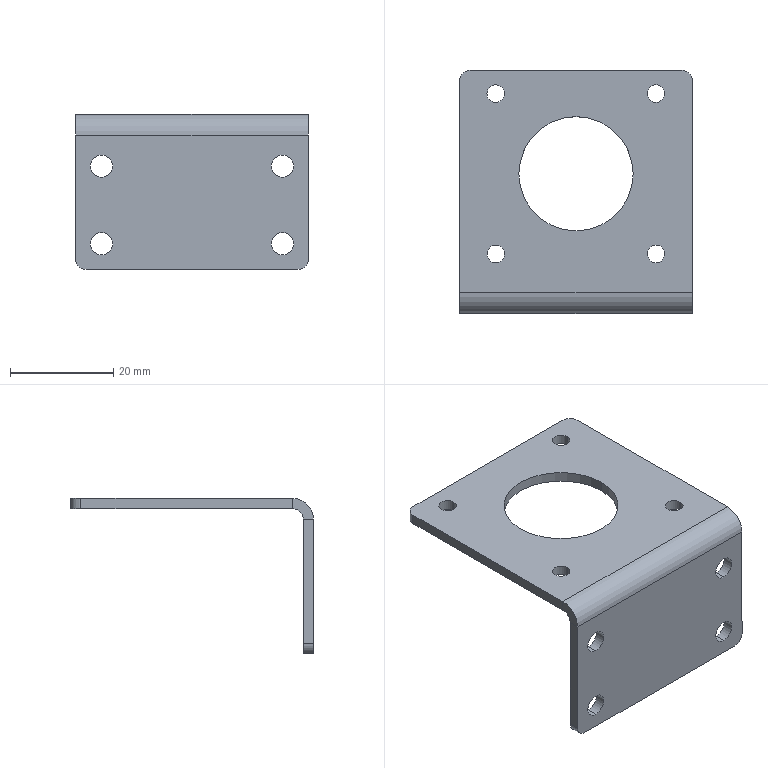Part | SolidWorks | features 3DProfileFeature 2, HoleWzd 2, EdgeFlange 1, Fillet 1, FlatPattern 1, ICE 1, SMBaseFlange 1, SheetMetal 1 | 1 solid | 36 faces | box 45 x 47 x 30 mm | volume 5671 mm3 | cylinder 24 | plane 12 | commonest cylinder face diameters 3.4 x8 4.3 x8 4 x5 22.1 x2 8 x1
STEP:
#1=CARTESIAN_POINT('',(-17.5,-23.5,-27.15));
#2=VERTEX_POINT('',#1);
#3=CARTESIAN_POINT('',(-17.5,-23.5,-22.85));
#4=VERTEX_POINT('',#3);
#5=CARTESIAN_POINT('',(-17.5,-23.5,-25.));
#6=DIRECTION('',(0.,1.,0.));
#7=DIRECTION('',(0.,0.,1.));
#8=AXIS2_PLACEMENT_3D('',#5,#6,#7);
#9=CIRCLE('',#8,2.15);
#10=EDGE_CURVE('',#2,#4,#9,.T.);
#11=ORIENTED_EDGE('',*,*,#10,.F.);
#12=CARTESIAN_POINT('',(-17.5,-21.5,-27.15));
#13=VERTEX_POINT('',#12);
#14=CARTESIAN_POINT('',(-17.5,-21.5,-27.15));
#15=DIRECTION('',(0.,1.,0.));
#16=VECTOR('',#15,1000.);
#17=LINE('',#14,#16);
#18=EDGE_CURVE('',#2,#13,#17,.T.);
#19=ORIENTED_EDGE('',*,*,#18,.T.);
#20=CARTESIAN_POINT('',(-17.5,-21.5,-22.85));
#21=VERTEX_POINT('',#20);
#22=CARTESIAN_POINT('',(-17.5,-21.5,-25.));
#23=DIRECTION('',(0.,1.,0.));
#24=DIRECTION('',(0.,0.,1.));
#25=AXIS2_PLACEMENT_3D('',#22,#23,#24);
#26=CIRCLE('',#25,2.15);
#27=EDGE_CURVE('',#13,#21,#26,.T.);
#28=ORIENTED_EDGE('',*,*,#27,.T.);
#29=CARTESIAN_POINT('',(-17.5,-21.5,-22.85));
#30=DIRECTION('',(0.,1.,0.));
#31=VECTOR('',#30,1000.);
#32=LINE('',#29,#31);
#33=EDGE_CURVE('',#4,#21,#32,.T.);
#34=ORIENTED_EDGE('',*,*,#33,.F.);
#35=EDGE_LOOP('',(#11,#19,#28,#34));
#36=FACE_OUTER_BOUND('',#35,.T.);
#37=CARTESIAN_POINT('',(-17.5,-21.5,-25.));
#38=DIRECTION('',(0.,1.,0.));
#39=DIRECTION('',(0.,0.,1.));
#40=AXIS2_PLACEMENT_3D('',#37,#38,#39);
#41=CYLINDRICAL_SURFACE('',#40,2.15);
#42=ADVANCED_FACE('',(#36),#41,.F.);
#43=CARTESIAN_POINT('',(-17.5,-23.5,-12.15));
#44=VERTEX_POINT('',#43);
#45=CARTESIAN_POINT('',(-17.5,-23.5,-7.85));
#46=VERTEX_POINT('',#45);
#47=CARTESIAN_POINT('',(-17.5,-23.5,-10.));
#48=DIRECTION('',(0.,1.,0.));
#49=DIRECTION('',(0.,0.,1.));
#50=AXIS2_PLACEMENT_3D('',#47,#48,#49);
#51=CIRCLE('',#50,2.15);
#52=EDGE_CURVE('',#44,#46,#51,.T.);
#53=ORIENTED_EDGE('',*,*,#52,.F.);
#54=CARTESIAN_POINT('',(-17.5,-21.5,-12.15));
#55=VERTEX_POINT('',#54);
#56=CARTESIAN_POINT('',(-17.5,-21.5,-12.15));
#57=DIRECTION('',(0.,1.,0.));
#58=VECTOR('',#57,1000.);
#59=LINE('',#56,#58);
#60=EDGE_CURVE('',#44,#55,#59,.T.);
#61=ORIENTED_EDGE('',*,*,#60,.T.);
#62=CARTESIAN_POINT('',(-17.5,-21.5,-7.85));
#63=VERTEX_POINT('',#62);
#64=CARTESIAN_POINT('',(-17.5,-21.5,-10.));
#65=DIRECTION('',(0.,1.,0.));
#66=DIRECTION('',(0.,0.,1.));
#67=AXIS2_PLACEMENT_3D('',#64,#65,#66);
#68=CIRCLE('',#67,2.15);
#69=EDGE_CURVE('',#55,#63,#68,.T.);
#70=ORIENTED_EDGE('',*,*,#69,.T.);
#71=CARTESIAN_POINT('',(-17.5,-21.5,-7.85));
#72=DIRECTION('',(0.,1.,0.));
#73=VECTOR('',#72,1000.);
#74=LINE('',#71,#73);
#75=EDGE_CURVE('',#46,#63,#74,.T.);
#76=ORIENTED_EDGE('',*,*,#75,.F.);
#77=EDGE_LOOP('',(#53,#61,#70,#76));
#78=FACE_OUTER_BOUND('',#77,.T.);
#79=CARTESIAN_POINT('',(-17.5,-21.5,-10.));
#80=DIRECTION('',(0.,1.,0.));
#81=DIRECTION('',(0.,0.,1.));
#82=AXIS2_PLACEMENT_3D('',#79,#80,#81);
#83=CYLINDRICAL_SURFACE('',#82,2.15);
#84=ADVANCED_FACE('',(#78),#83,.F.);
#85=CARTESIAN_POINT('',(17.5,-23.5,-27.15));
#86=VERTEX_POINT('',#85);
#87=CARTESIAN_POINT('',(17.5,-23.5,-22.85));
#88=VERTEX_POINT('',#87);
#89=CARTESIAN_POINT('',(17.5,-23.5,-25.));
#90=DIRECTION('',(0.,1.,0.));
#91=DIRECTION('',(0.,0.,1.));
#92=AXIS2_PLACEMENT_3D('',#89,#90,#91);
#93=CIRCLE('',#92,2.15);
#94=EDGE_CURVE('',#86,#88,#93,.T.);
#95=ORIENTED_EDGE('',*,*,#94,.F.);
#96=CARTESIAN_POINT('',(17.5,-21.5,-27.15));
#97=VERTEX_POINT('',#96);
#98=CARTESIAN_POINT('',(17.5,-21.5,-27.15));
#99=DIRECTION('',(0.,1.,0.));
#100=VECTOR('',#99,1000.);
#101=LINE('',#98,#100);
#102=EDGE_CURVE('',#86,#97,#101,.T.);
#103=ORIENTED_EDGE('',*,*,#102,.T.);
#104=CARTESIAN_POINT('',(17.5,-21.5,-22.85));
#105=VERTEX_POINT('',#104);
#106=CARTESIAN_POINT('',(17.5,-21.5,-25.));
#107=DIRECTION('',(0.,1.,0.));
#108=DIRECTION('',(0.,0.,1.));
#109=AXIS2_PLACEMENT_3D('',#106,#107,#108);
#110=CIRCLE('',#109,2.15);
#111=EDGE_CURVE('',#97,#105,#110,.T.);
#112=ORIENTED_EDGE('',*,*,#111,.T.);
#113=CARTESIAN_POINT('',(17.5,-21.5,-22.85));
#114=DIRECTION('',(0.,1.,0.));
#115=VECTOR('',#114,1000.);
#116=LINE('',#113,#115);
#117=EDGE_CURVE('',#88,#105,#116,.T.);
#118=ORIENTED_EDGE('',*,*,#117,.F.);
#119=EDGE_LOOP('',(#95,#103,#112,#118));
#120=FACE_OUTER_BOUND('',#119,.T.);
#121=CARTESIAN_POINT('',(17.5,-21.5,-25.));
#122=DIRECTION('',(0.,1.,0.));
#123=DIRECTION('',(0.,0.,1.));
#124=AXIS2_PLACEMENT_3D('',#121,#122,#123);
#125=CYLINDRICAL_SURFACE('',#124,2.15);
#126=ADVANCED_FACE('',(#120),#125,.F.);
#127=CARTESIAN_POINT('',(17.5,-23.5,-12.15));
#128=VERTEX_POINT('',#127);
#129=CARTESIAN_POINT('',(17.5,-23.5,-7.85));
#130=VERTEX_POINT('',#129);
#131=CARTESIAN_POINT('',(17.5,-23.5,-10.));
#132=DIRECTION('',(0.,1.,0.));
#133=DIRECTION('',(0.,0.,1.));
#134=AXIS2_PLACEMENT_3D('',#131,#132,#133);
#135=CIRCLE('',#134,2.15);
#136=EDGE_CURVE('',#128,#130,#135,.T.);
#137=ORIENTED_EDGE('',*,*,#136,.F.);
#138=CARTESIAN_POINT('',(17.5,-21.5,-12.15));
#139=VERTEX_POINT('',#138);
#140=CARTESIAN_POINT('',(17.5,-21.5,-12.15));
#141=DIRECTION('',(0.,1.,0.));
#142=VECTOR('',#141,1000.);
#143=LINE('',#140,#142);
#144=EDGE_CURVE('',#128,#139,#143,.T.);
#145=ORIENTED_EDGE('',*,*,#144,.T.);
#146=CARTESIAN_POINT('',(17.5,-21.5,-7.85));
#147=VERTEX_POINT('',#146);
#148=CARTESIAN_POINT('',(17.5,-21.5,-10.));
#149=DIRECTION('',(0.,1.,0.));
#150=DIRECTION('',(0.,0.,1.));
#151=AXIS2_PLACEMENT_3D('',#148,#149,#150);
#152=CIRCLE('',#151,2.15);
#153=EDGE_CURVE('',#139,#147,#152,.T.);
#154=ORIENTED_EDGE('',*,*,#153,.T.);
#155=CARTESIAN_POINT('',(17.5,-21.5,-7.85));
#156=DIRECTION('',(0.,1.,0.));
#157=VECTOR('',#156,1000.);
#158=LINE('',#155,#157);
#159=EDGE_CURVE('',#130,#147,#158,.T.);
#160=ORIENTED_EDGE('',*,*,#159,.F.);
#161=EDGE_LOOP('',(#137,#145,#154,#160));
#162=FACE_OUTER_BOUND('',#161,.T.);
#163=CARTESIAN_POINT('',(17.5,-21.5,-10.));
#164=DIRECTION('',(0.,1.,0.));
#165=DIRECTION('',(0.,0.,1.));
#166=AXIS2_PLACEMENT_3D('',#163,#164,#165);
#167=CYLINDRICAL_SURFACE('',#166,2.15);
#168=ADVANCED_FACE('',(#162),#167,.F.);
#169=CARTESIAN_POINT('',(-13.804,-12.003,-2.));
#170=VERTEX_POINT('',#169);
#171=CARTESIAN_POINT('',(-17.204,-12.003,-2.));
#172=VERTEX_POINT('',#171);
#173=CARTESIAN_POINT('',(-15.504,-12.003,-2.));
#174=DIRECTION('',(0.,0.,-1.));
#175=DIRECTION('',(-1.,0.,0.));
#176=AXIS2_PLACEMENT_3D('',#173,#174,#175);
#177=CIRCLE('',#176,1.7);
#178=EDGE_CURVE('',#170,#172,#177,.T.);
#179=ORIENTED_EDGE('',*,*,#178,.T.);
#180=CARTESIAN_POINT('',(-17.204,-12.003,0.));
#181=VERTEX_POINT('',#180);
#182=CARTESIAN_POINT('',(-17.204,-12.003,0.));
#183=DIRECTION('',(0.,0.,1.));
#184=VECTOR('',#183,1000.);
#185=LINE('',#182,#184);
#186=EDGE_CURVE('',#172,#181,#185,.T.);
#187=ORIENTED_EDGE('',*,*,#186,.T.);
#188=CARTESIAN_POINT('',(-13.804,-12.003,0.));
#189=VERTEX_POINT('',#188);
#190=CARTESIAN_POINT('',(-15.504,-12.003,0.));
#191=DIRECTION('',(0.,0.,1.));
#192=DIRECTION('',(1.,0.,0.));
#193=AXIS2_PLACEMENT_3D('',#190,#191,#192);
#194=CIRCLE('',#193,1.7);
#195=EDGE_CURVE('',#181,#189,#194,.T.);
#196=ORIENTED_EDGE('',*,*,#195,.T.);
#197=CARTESIAN_POINT('',(-13.804,-12.003,0.));
#198=DIRECTION('',(0.,0.,1.));
#199=VECTOR('',#198,1000.);
#200=LINE('',#197,#199);
#201=EDGE_CURVE('',#170,#189,#200,.T.);
#202=ORIENTED_EDGE('',*,*,#201,.F.);
#203=EDGE_LOOP('',(#179,#187,#196,#202));
#204=FACE_OUTER_BOUND('',#203,.T.);
#205=CARTESIAN_POINT('',(-15.504,-12.003,0.));
#206=DIRECTION('',(0.,0.,1.));
#207=DIRECTION('',(1.,0.,0.));
#208=AXIS2_PLACEMENT_3D('',#205,#206,#207);
#209=CYLINDRICAL_SURFACE('',#208,1.7);
#210=ADVANCED_FACE('',(#204),#209,.F.);
#211=CARTESIAN_POINT('',(17.182,-11.997,-2.));
#212=VERTEX_POINT('',#211);
#213=CARTESIAN_POINT('',(13.782,-11.997,-2.));
#214=VERTEX_POINT('',#213);
#215=CARTESIAN_POINT('',(15.482,-11.997,-2.));
#216=DIRECTION('',(0.,0.,-1.));
#217=DIRECTION('',(-1.,0.,0.));
#218=AXIS2_PLACEMENT_3D('',#215,#216,#217);
#219=CIRCLE('',#218,1.7);
#220=EDGE_CURVE('',#212,#214,#219,.T.);
#221=ORIENTED_EDGE('',*,*,#220,.T.);
#222=CARTESIAN_POINT('',(13.782,-11.997,0.));
#223=VERTEX_POINT('',#222);
#224=CARTESIAN_POINT('',(13.782,-11.997,0.));
#225=DIRECTION('',(0.,0.,1.));
#226=VECTOR('',#225,1000.);
#227=LINE('',#224,#226);
#228=EDGE_CURVE('',#214,#223,#227,.T.);
#229=ORIENTED_EDGE('',*,*,#228,.T.);
#230=CARTESIAN_POINT('',(17.182,-11.997,0.));
#231=VERTEX_POINT('',#230);
#232=CARTESIAN_POINT('',(15.482,-11.997,0.));
#233=DIRECTION('',(0.,0.,1.));
#234=DIRECTION('',(1.,0.,0.));
#235=AXIS2_PLACEMENT_3D('',#232,#233,#234);
#236=CIRCLE('',#235,1.7);
#237=EDGE_CURVE('',#223,#231,#236,.T.);
#238=ORIENTED_EDGE('',*,*,#237,.T.);
#239=CARTESIAN_POINT('',(17.182,-11.997,0.));
#240=DIRECTION('',(0.,0.,1.));
#241=VECTOR('',#240,1000.);
#242=LINE('',#239,#241);
#243=EDGE_CURVE('',#212,#231,#242,.T.);
#244=ORIENTED_EDGE('',*,*,#243,.F.);
#245=EDGE_LOOP('',(#221,#229,#238,#244));
#246=FACE_OUTER_BOUND('',#245,.T.);
#247=CARTESIAN_POINT('',(15.482,-11.997,0.));
#248=DIRECTION('',(0.,0.,1.));
#249=DIRECTION('',(1.,0.,0.));
#250=AXIS2_PLACEMENT_3D('',#247,#248,#249);
#251=CYLINDRICAL_SURFACE('',#250,1.7);
#252=ADVANCED_FACE('',(#246),#251,.F.);
#253=CARTESIAN_POINT('',(17.167,18.994,-2.));
#254=VERTEX_POINT('',#253);
#255=CARTESIAN_POINT('',(13.767,18.994,-2.));
#256=VERTEX_POINT('',#255);
#257=CARTESIAN_POINT('',(15.467,18.994,-2.));
#258=DIRECTION('',(0.,0.,-1.));
#259=DIRECTION('',(-1.,0.,0.));
#260=AXIS2_PLACEMENT_3D('',#257,#258,#259);
#261=CIRCLE('',#260,1.7);
#262=EDGE_CURVE('',#254,#256,#261,.T.);
#263=ORIENTED_EDGE('',*,*,#262,.T.);
#264=CARTESIAN_POINT('',(13.767,18.994,0.));
#265=VERTEX_POINT('',#264);
#266=CARTESIAN_POINT('',(13.767,18.994,0.));
#267=DIRECTION('',(0.,0.,1.));
#268=VECTOR('',#267,1000.);
#269=LINE('',#266,#268);
#270=EDGE_CURVE('',#256,#265,#269,.T.);
#271=ORIENTED_EDGE('',*,*,#270,.T.);
#272=CARTESIAN_POINT('',(17.167,18.994,0.));
#273=VERTEX_POINT('',#272);
#274=CARTESIAN_POINT('',(15.467,18.994,0.));
#275=DIRECTION('',(0.,0.,1.));
#276=DIRECTION('',(1.,0.,0.));
#277=AXIS2_PLACEMENT_3D('',#274,#275,#276);
#278=CIRCLE('',#277,1.7);
#279=EDGE_CURVE('',#265,#273,#278,.T.);
#280=ORIENTED_EDGE('',*,*,#279,.T.);
#281=CARTESIAN_POINT('',(17.167,18.994,0.));
#282=DIRECTION('',(0.,0.,1.));
#283=VECTOR('',#282,1000.);
#284=LINE('',#281,#283);
#285=EDGE_CURVE('',#254,#273,#284,.T.);
#286=ORIENTED_EDGE('',*,*,#285,.F.);
#287=EDGE_LOOP('',(#263,#271,#280,#286));
#288=FACE_OUTER_BOUND('',#287,.T.);
#289=CARTESIAN_POINT('',(15.467,18.994,0.));
#290=DIRECTION('',(0.,0.,1.));
#291=DIRECTION('',(1.,0.,0.));
#292=AXIS2_PLACEMENT_3D('',#289,#290,#291);
#293=CYLINDRICAL_SURFACE('',#292,1.7);
#294=ADVANCED_FACE('',(#288),#293,.F.);
#295=CARTESIAN_POINT('',(-13.822,18.991,-2.));
#296=VERTEX_POINT('',#295);
#297=CARTESIAN_POINT('',(-17.222,18.991,-2.));
#298=VERTEX_POINT('',#297);
#299=CARTESIAN_POINT('',(-15.522,18.991,-2.));
#300=DIRECTION('',(0.,0.,-1.));
#301=DIRECTION('',(-1.,0.,0.));
#302=AXIS2_PLACEMENT_3D('',#299,#300,#301);
#303=CIRCLE('',#302,1.7);
#304=EDGE_CURVE('',#296,#298,#303,.T.);
#305=ORIENTED_EDGE('',*,*,#304,.T.);
#306=CARTESIAN_POINT('',(-17.222,18.991,0.));
#307=VERTEX_POINT('',#306);
#308=CARTESIAN_POINT('',(-17.222,18.991,0.));
#309=DIRECTION('',(0.,0.,1.));
#310=VECTOR('',#309,1000.);
#311=LINE('',#308,#310);
#312=EDGE_CURVE('',#298,#307,#311,.T.);
#313=ORIENTED_EDGE('',*,*,#312,.T.);
#314=CARTESIAN_POINT('',(-13.822,18.991,0.));
#315=VERTEX_POINT('',#314);
#316=CARTESIAN_POINT('',(-15.522,18.991,0.));
#317=DIRECTION('',(0.,0.,1.));
#318=DIRECTION('',(1.,0.,0.));
#319=AXIS2_PLACEMENT_3D('',#316,#317,#318);
#320=CIRCLE('',#319,1.7);
#321=EDGE_CURVE('',#307,#315,#320,.T.);
#322=ORIENTED_EDGE('',*,*,#321,.T.);
#323=CARTESIAN_POINT('',(-13.822,18.991,0.));
#324=DIRECTION('',(0.,0.,1.));
#325=VECTOR('',#324,1000.);
#326=LINE('',#323,#325);
#327=EDGE_CURVE('',#296,#315,#326,.T.);
#328=ORIENTED_EDGE('',*,*,#327,.F.);
#329=EDGE_LOOP('',(#305,#313,#322,#328));
#330=FACE_OUTER_BOUND('',#329,.T.);
#331=CARTESIAN_POINT('',(-15.522,18.991,0.));
#332=DIRECTION('',(0.,0.,1.));
#333=DIRECTION('',(1.,0.,0.));
#334=AXIS2_PLACEMENT_3D('',#331,#332,#333);
#335=CYLINDRICAL_SURFACE('',#334,1.7);
#336=ADVANCED_FACE('',(#330),#335,.F.);
#337=CARTESIAN_POINT('',(11.05,3.5,-2.));
#338=VERTEX_POINT('',#337);
#339=CARTESIAN_POINT('',(-11.05,3.5,-2.));
#340=VERTEX_POINT('',#339);
#341=CARTESIAN_POINT('',(0.,3.5,-2.));
#342=DIRECTION('',(0.,0.,-1.));
#343=DIRECTION('',(-1.,0.,0.));
#344=AXIS2_PLACEMENT_3D('',#341,#342,#343);
#345=CIRCLE('',#344,11.05);
#346=EDGE_CURVE('',#338,#340,#345,.T.);
#347=ORIENTED_EDGE('',*,*,#346,.T.);
#348=CARTESIAN_POINT('',(-11.05,3.5,0.));
#349=VERTEX_POINT('',#348);
#350=CARTESIAN_POINT('',(-11.05,3.5,-30.));
#351=DIRECTION('',(0.,0.,1.));
#352=VECTOR('',#351,1000.);
#353=LINE('',#350,#352);
#354=EDGE_CURVE('',#340,#349,#353,.T.);
#355=ORIENTED_EDGE('',*,*,#354,.T.);
#356=CARTESIAN_POINT('',(11.05,3.5,0.));
#357=VERTEX_POINT('',#356);
#358=CARTESIAN_POINT('',(0.,3.5,0.));
#359=DIRECTION('',(0.,0.,1.));
#360=DIRECTION('',(1.,0.,0.));
#361=AXIS2_PLACEMENT_3D('',#358,#359,#360);
#362=CIRCLE('',#361,11.05);
#363=EDGE_CURVE('',#349,#357,#362,.T.);
#364=ORIENTED_EDGE('',*,*,#363,.T.);
#365=CARTESIAN_POINT('',(11.05,3.5,-30.));
#366=DIRECTION('',(0.,0.,1.));
#367=VECTOR('',#366,1000.);
#368=LINE('',#365,#367);
#369=EDGE_CURVE('',#338,#357,#368,.T.);
#370=ORIENTED_EDGE('',*,*,#369,.F.);
#371=EDGE_LOOP('',(#347,#355,#364,#370));
#372=FACE_OUTER_BOUND('',#371,.T.);
#373=CARTESIAN_POINT('',(0.,3.5,-30.));
#374=DIRECTION('',(0.,0.,1.));
#375=DIRECTION('',(1.,0.,0.));
#376=AXIS2_PLACEMENT_3D('',#373,#374,#375);
#377=CYLINDRICAL_SURFACE('',#376,11.05);
#378=ADVANCED_FACE('',(#372),#377,.F.);
#379=CARTESIAN_POINT('',(-22.5,-23.5,-28.));
#380=VERTEX_POINT('',#379);
#381=CARTESIAN_POINT('',(-22.5,-23.5,-4.));
#382=VERTEX_POINT('',#381);
#383=CARTESIAN_POINT('',(-22.5,-23.5,-2.));
#384=DIRECTION('',(0.,0.,1.));
#385=VECTOR('',#384,1000.);
#386=LINE('',#383,#385);
#387=EDGE_CURVE('',#380,#382,#386,.T.);
#388=ORIENTED_EDGE('',*,*,#387,.F.);
#389=CARTESIAN_POINT('',(-20.5,-23.5,-30.));
#390=VERTEX_POINT('',#389);
#391=CARTESIAN_POINT('',(-20.5,-23.5,-28.));
#392=DIRECTION('',(0.,-1.,0.));
#393=DIRECTION('',(0.,0.,-1.));
#394=AXIS2_PLACEMENT_3D('',#391,#392,#393);
#395=CIRCLE('',#394,2.);
#396=EDGE_CURVE('',#380,#390,#395,.T.);
#397=ORIENTED_EDGE('',*,*,#396,.T.);
#398=CARTESIAN_POINT('',(20.5,-23.5,-30.));
#399=VERTEX_POINT('',#398);
#400=CARTESIAN_POINT('',(-22.5,-23.5,-30.));
#401=DIRECTION('',(-1.,0.,0.));
#402=VECTOR('',#401,1000.);
#403=LINE('',#400,#402);
#404=EDGE_CURVE('',#399,#390,#403,.T.);
#405=ORIENTED_EDGE('',*,*,#404,.F.);
#406=CARTESIAN_POINT('',(22.5,-23.5,-28.));
#407=VERTEX_POINT('',#406);
#408=CARTESIAN_POINT('',(20.5,-23.5,-28.));
#409=DIRECTION('',(0.,-1.,0.));
#410=DIRECTION('',(0.,0.,-1.));
#411=AXIS2_PLACEMENT_3D('',#408,#409,#410);
#412=CIRCLE('',#411,2.);
#413=EDGE_CURVE('',#399,#407,#412,.T.);
#414=ORIENTED_EDGE('',*,*,#413,.T.);
#415=CARTESIAN_POINT('',(22.5,-23.5,-4.));
#416=VERTEX_POINT('',#415);
#417=CARTESIAN_POINT('',(22.5,-23.5,-30.));
#418=DIRECTION('',(0.,0.,-1.));
#419=VECTOR('',#418,1000.);
#420=LINE('',#417,#419);
#421=EDGE_CURVE('',#416,#407,#420,.T.);
#422=ORIENTED_EDGE('',*,*,#421,.F.);
#423=CARTESIAN_POINT('',(0.,-23.5,-4.));
#424=DIRECTION('',(-1.,0.,0.));
#425=VECTOR('',#424,1000.);
#426=LINE('',#423,#425);
#427=EDGE_CURVE('',#416,#382,#426,.T.);
#428=ORIENTED_EDGE('',*,*,#427,.T.);
#429=EDGE_LOOP('',(#388,#397,#405,#414,#422,#428));
#430=FACE_OUTER_BOUND('',#429,.T.);
#431=CARTESIAN_POINT('',(17.5,-23.5,-10.));
#432=DIRECTION('',(0.,1.,0.));
#433=DIRECTION('',(0.,0.,1.));
#434=AXIS2_PLACEMENT_3D('',#431,#432,#433);
#435=CIRCLE('',#434,2.15);
#436=EDGE_CURVE('',#130,#128,#435,.T.);
#437=ORIENTED_EDGE('',*,*,#436,.T.);
#438=ORIENTED_EDGE('',*,*,#136,.T.);
#439=EDGE_LOOP('',(#437,#438));
#440=FACE_BOUND('',#439,.T.);
#441=CARTESIAN_POINT('',(17.5,-23.5,-25.));
#442=DIRECTION('',(0.,1.,0.));
#443=DIRECTION('',(0.,0.,1.));
#444=AXIS2_PLACEMENT_3D('',#441,#442,#443);
#445=CIRCLE('',#444,2.15);
#446=EDGE_CURVE('',#88,#86,#445,.T.);
#447=ORIENTED_EDGE('',*,*,#446,.T.);
#448=ORIENTED_EDGE('',*,*,#94,.T.);
#449=EDGE_LOOP('',(#447,#448));
#450=FACE_BOUND('',#449,.T.);
#451=CARTESIAN_POINT('',(-17.5,-23.5,-10.));
#452=DIRECTION('',(0.,1.,0.));
#453=DIRECTION('',(0.,0.,1.));
#454=AXIS2_PLACEMENT_3D('',#451,#452,#453);
#455=CIRCLE('',#454,2.15);
#456=EDGE_CURVE('',#46,#44,#455,.T.);
#457=ORIENTED_EDGE('',*,*,#456,.T.);
#458=ORIENTED_EDGE('',*,*,#52,.T.);
#459=EDGE_LOOP('',(#457,#458));
#460=FACE_BOUND('',#459,.T.);
#461=CARTESIAN_POINT('',(-17.5,-23.5,-25.));
#462=DIRECTION('',(0.,1.,0.));
#463=DIRECTION('',(0.,0.,1.));
#464=AXIS2_PLACEMENT_3D('',#461,#462,#463);
#465=CIRCLE('',#464,2.15);
#466=EDGE_CURVE('',#4,#2,#465,.T.);
#467=ORIENTED_EDGE('',*,*,#466,.T.);
#468=ORIENTED_EDGE('',*,*,#10,.T.);
#469=EDGE_LOOP('',(#467,#468));
#470=FACE_BOUND('',#469,.T.);
#471=CARTESIAN_POINT('',(0.,-23.5,0.));
#472=DIRECTION('',(0.,-1.,0.));
#473=DIRECTION('',(0.,0.,-1.));
#474=AXIS2_PLACEMENT_3D('',#471,#472,#473);
#475=PLANE('',#474);
#476=ADVANCED_FACE('',(#430,#440,#450,#460,#470),#475,.T.);
#477=CARTESIAN_POINT('',(-17.5,-21.5,-10.));
#478=DIRECTION('',(0.,1.,0.));
#479=DIRECTION('',(0.,0.,1.));
#480=AXIS2_PLACEMENT_3D('',#477,#478,#479);
#481=CIRCLE('',#480,2.15);
#482=EDGE_CURVE('',#63,#55,#481,.T.);
#483=ORIENTED_EDGE('',*,*,#482,.F.);
#484=ORIENTED_EDGE('',*,*,#69,.F.);
#485=EDGE_LOOP('',(#483,#484));
#486=FACE_BOUND('',#485,.T.);
#487=CARTESIAN_POINT('',(17.5,-21.5,-25.));
#488=DIRECTION('',(0.,1.,0.));
#489=DIRECTION('',(0.,0.,1.));
#490=AXIS2_PLACEMENT_3D('',#487,#488,#489);
#491=CIRCLE('',#490,2.15);
#492=EDGE_CURVE('',#105,#97,#491,.T.);
#493=ORIENTED_EDGE('',*,*,#492,.F.);
#494=ORIENTED_EDGE('',*,*,#111,.F.);
#495=EDGE_LOOP('',(#493,#494));
#496=FACE_BOUND('',#495,.T.);
#497=CARTESIAN_POINT('',(17.5,-21.5,-10.));
#498=DIRECTION('',(0.,1.,0.));
#499=DIRECTION('',(0.,0.,1.));
#500=AXIS2_PLACEMENT_3D('',#497,#498,#499);
#501=CIRCLE('',#500,2.15);
#502=EDGE_CURVE('',#147,#139,#501,.T.);
#503=ORIENTED_EDGE('',*,*,#502,.F.);
#504=ORIENTED_EDGE('',*,*,#153,.F.);
#505=EDGE_LOOP('',(#503,#504));
#506=FACE_BOUND('',#505,.T.);
#507=CARTESIAN_POINT('',(20.5,-21.5,-30.));
#508=VERTEX_POINT('',#507);
#509=CARTESIAN_POINT('',(-20.5,-21.5,-30.));
#510=VERTEX_POINT('',#509);
#511=CARTESIAN_POINT('',(0.,-21.5,-30.));
#512=DIRECTION('',(-1.,0.,0.));
#513=VECTOR('',#512,1000.);
#514=LINE('',#511,#513);
#515=EDGE_CURVE('',#508,#510,#514,.T.);
#516=ORIENTED_EDGE('',*,*,#515,.T.);
#517=CARTESIAN_POINT('',(-22.5,-21.5,-28.));
#518=VERTEX_POINT('',#517);
#519=CARTESIAN_POINT('',(-20.5,-21.5,-28.));
#520=DIRECTION('',(0.,1.,0.));
#521=DIRECTION('',(0.,0.,-1.));
#522=AXIS2_PLACEMENT_3D('',#519,#520,#521);
#523=CIRCLE('',#522,2.);
#524=EDGE_CURVE('',#510,#518,#523,.T.);
#525=ORIENTED_EDGE('',*,*,#524,.T.);
#526=CARTESIAN_POINT('',(-22.5,-21.5,-4.));
#527=VERTEX_POINT('',#526);
#528=CARTESIAN_POINT('',(-22.5,-21.5,0.));
#529=DIRECTION('',(0.,0.,1.));
#530=VECTOR('',#529,1000.);
#531=LINE('',#528,#530);
#532=EDGE_CURVE('',#518,#527,#531,.T.);
#533=ORIENTED_EDGE('',*,*,#532,.T.);
#534=CARTESIAN_POINT('',(22.5,-21.5,-4.));
#535=VERTEX_POINT('',#534);
#536=CARTESIAN_POINT('',(22.5,-21.5,-4.));
#537=DIRECTION('',(-1.,0.,0.));
#538=VECTOR('',#537,1000.);
#539=LINE('',#536,#538);
#540=EDGE_CURVE('',#535,#527,#539,.T.);
#541=ORIENTED_EDGE('',*,*,#540,.F.);
#542=CARTESIAN_POINT('',(22.5,-21.5,-28.));
#543=VERTEX_POINT('',#542);
#544=CARTESIAN_POINT('',(22.5,-21.5,0.));
#545=DIRECTION('',(0.,0.,-1.));
#546=VECTOR('',#545,1000.);
#547=LINE('',#544,#546);
#548=EDGE_CURVE('',#535,#543,#547,.T.);
#549=ORIENTED_EDGE('',*,*,#548,.T.);
#550=CARTESIAN_POINT('',(20.5,-21.5,-28.));
#551=DIRECTION('',(0.,1.,0.));
#552=DIRECTION('',(0.,0.,-1.));
#553=AXIS2_PLACEMENT_3D('',#550,#551,#552);
#554=CIRCLE('',#553,2.);
#555=EDGE_CURVE('',#543,#508,#554,.T.);
#556=ORIENTED_EDGE('',*,*,#555,.T.);
#557=EDGE_LOOP('',(#516,#525,#533,#541,#549,#556));
#558=FACE_OUTER_BOUND('',#557,.T.);
#559=CARTESIAN_POINT('',(-17.5,-21.5,-25.));
#560=DIRECTION('',(0.,1.,0.));
#561=DIRECTION('',(0.,0.,1.));
#562=AXIS2_PLACEMENT_3D('',#559,#560,#561);
#563=CIRCLE('',#562,2.15);
#564=EDGE_CURVE('',#21,#13,#563,.T.);
#565=ORIENTED_EDGE('',*,*,#564,.F.);
#566=ORIENTED_EDGE('',*,*,#27,.F.);
#567=EDGE_LOOP('',(#565,#566));
#568=FACE_BOUND('',#567,.T.);
#569=CARTESIAN_POINT('',(0.,-21.5,0.));
#570=DIRECTION('',(0.,-1.,0.));
#571=DIRECTION('',(0.,0.,-1.));
#572=AXIS2_PLACEMENT_3D('',#569,#570,#571);
#573=PLANE('',#572);
#574=ADVANCED_FACE('',(#486,#496,#506,#558,#568),#573,.F.);
#575=CARTESIAN_POINT('',(-22.5,21.5,0.));
#576=VERTEX_POINT('',#575);
#577=CARTESIAN_POINT('',(-22.5,-19.5,0.));
#578=VERTEX_POINT('',#577);
#579=CARTESIAN_POINT('',(-22.5,-23.5,0.));
#580=DIRECTION('',(0.,-1.,0.));
#581=VECTOR('',#580,1000.);
#582=LINE('',#579,#581);
#583=EDGE_CURVE('',#576,#578,#582,.T.);
#584=ORIENTED_EDGE('',*,*,#583,.F.);
#585=CARTESIAN_POINT('',(-22.5,21.5,-2.));
#586=VERTEX_POINT('',#585);
#587=CARTESIAN_POINT('',(-22.5,21.5,-2.));
#588=DIRECTION('',(0.,0.,-1.));
#589=VECTOR('',#588,1000.);
#590=LINE('',#587,#589);
#591=EDGE_CURVE('',#576,#586,#590,.T.);
#592=ORIENTED_EDGE('',*,*,#591,.T.);
#593=CARTESIAN_POINT('',(-22.5,-19.5,-2.));
#594=VERTEX_POINT('',#593);
#595=CARTESIAN_POINT('',(-22.5,-23.5,-2.));
#596=DIRECTION('',(0.,-1.,0.));
#597=VECTOR('',#596,1000.);
#598=LINE('',#595,#597);
#599=EDGE_CURVE('',#586,#594,#598,.T.);
#600=ORIENTED_EDGE('',*,*,#599,.T.);
#601=CARTESIAN_POINT('',(-22.5,-19.5,-2.));
#602=DIRECTION('',(0.,0.,1.));
#603=VECTOR('',#602,1000.);
#604=LINE('',#601,#603);
#605=EDGE_CURVE('',#594,#578,#604,.T.);
#606=ORIENTED_EDGE('',*,*,#605,.T.);
#607=EDGE_LOOP('',(#584,#592,#600,#606));
#608=FACE_OUTER_BOUND('',#607,.T.);
#609=CARTESIAN_POINT('',(-22.5,-23.5,-2.));
#610=DIRECTION('',(-1.,0.,0.));
#611=DIRECTION('',(0.,0.,1.));
#612=AXIS2_PLACEMENT_3D('',#609,#610,#611);
#613=PLANE('',#612);
#614=ADVANCED_FACE('',(#608),#613,.T.);
#615=ORIENTED_EDGE('',*,*,#178,.F.);
#616=CARTESIAN_POINT('',(-15.504,-12.003,-2.));
#617=DIRECTION('',(0.,0.,-1.));
#618=DIRECTION('',(-1.,0.,0.));
#619=AXIS2_PLACEMENT_3D('',#616,#617,#618);
#620=CIRCLE('',#619,1.7);
#621=EDGE_CURVE('',#172,#170,#620,.T.);
#622=ORIENTED_EDGE('',*,*,#621,.F.);
#623=EDGE_LOOP('',(#615,#622));
#624=FACE_BOUND('',#623,.T.);
#625=ORIENTED_EDGE('',*,*,#220,.F.);
#626=CARTESIAN_POINT('',(15.482,-11.997,-2.));
#627=DIRECTION('',(0.,0.,-1.));
#628=DIRECTION('',(-1.,0.,0.));
#629=AXIS2_PLACEMENT_3D('',#626,#627,#628);
#630=CIRCLE('',#629,1.7);
#631=EDGE_CURVE('',#214,#212,#630,.T.);
#632=ORIENTED_EDGE('',*,*,#631,.F.);
#633=EDGE_LOOP('',(#625,#632));
#634=FACE_BOUND('',#633,.T.);
#635=ORIENTED_EDGE('',*,*,#262,.F.);
#636=CARTESIAN_POINT('',(15.467,18.994,-2.));
#637=DIRECTION('',(0.,0.,-1.));
#638=DIRECTION('',(-1.,0.,0.));
#639=AXIS2_PLACEMENT_3D('',#636,#637,#638);
#640=CIRCLE('',#639,1.7);
#641=EDGE_CURVE('',#256,#254,#640,.T.);
#642=ORIENTED_EDGE('',*,*,#641,.F.);
#643=EDGE_LOOP('',(#635,#642));
#644=FACE_BOUND('',#643,.T.);
#645=ORIENTED_EDGE('',*,*,#304,.F.);
#646=CARTESIAN_POINT('',(-15.522,18.991,-2.));
#647=DIRECTION('',(0.,0.,-1.));
#648=DIRECTION('',(-1.,0.,0.));
#649=AXIS2_PLACEMENT_3D('',#646,#647,#648);
#650=CIRCLE('',#649,1.7);
#651=EDGE_CURVE('',#298,#296,#650,.T.);
#652=ORIENTED_EDGE('',*,*,#651,.F.);
#653=EDGE_LOOP('',(#645,#652));
#654=FACE_BOUND('',#653,.T.);
#655=ORIENTED_EDGE('',*,*,#346,.F.);
#656=CARTESIAN_POINT('',(0.,3.5,-2.));
#657=DIRECTION('',(0.,0.,-1.));
#658=DIRECTION('',(-1.,0.,0.));
#659=AXIS2_PLACEMENT_3D('',#656,#657,#658);
#660=CIRCLE('',#659,11.05);
#661=EDGE_CURVE('',#340,#338,#660,.T.);
#662=ORIENTED_EDGE('',*,*,#661,.F.);
#663=EDGE_LOOP('',(#655,#662));
#664=FACE_BOUND('',#663,.T.);
#665=ORIENTED_EDGE('',*,*,#599,.F.);
#666=CARTESIAN_POINT('',(-20.5,23.5,-2.));
#667=VERTEX_POINT('',#666);
#668=CARTESIAN_POINT('',(-20.5,21.5,-2.));
#669=DIRECTION('',(0.,0.,-1.));
#670=DIRECTION('',(-1.,0.,0.));
#671=AXIS2_PLACEMENT_3D('',#668,#669,#670);
#672=CIRCLE('',#671,2.);
#673=EDGE_CURVE('',#586,#667,#672,.T.);
#674=ORIENTED_EDGE('',*,*,#673,.T.);
#675=CARTESIAN_POINT('',(20.5,23.5,-2.));
#676=VERTEX_POINT('',#675);
#677=CARTESIAN_POINT('',(-22.5,23.5,-2.));
#678=DIRECTION('',(-1.,0.,0.));
#679=VECTOR('',#678,1000.);
#680=LINE('',#677,#679);
#681=EDGE_CURVE('',#676,#667,#680,.T.);
#682=ORIENTED_EDGE('',*,*,#681,.F.);
#683=CARTESIAN_POINT('',(22.5,21.5,-2.));
#684=VERTEX_POINT('',#683);
#685=CARTESIAN_POINT('',(20.5,21.5,-2.));
#686=DIRECTION('',(0.,0.,-1.));
#687=DIRECTION('',(-1.,0.,0.));
#688=AXIS2_PLACEMENT_3D('',#685,#686,#687);
#689=CIRCLE('',#688,2.);
#690=EDGE_CURVE('',#676,#684,#689,.T.);
#691=ORIENTED_EDGE('',*,*,#690,.T.);
#692=CARTESIAN_POINT('',(22.5,-19.5,-2.));
#693=VERTEX_POINT('',#692);
#694=CARTESIAN_POINT('',(22.5,-23.5,-2.));
#695=DIRECTION('',(0.,1.,0.));
#696=VECTOR('',#695,1000.);
#697=LINE('',#694,#696);
#698=EDGE_CURVE('',#693,#684,#697,.T.);
#699=ORIENTED_EDGE('',*,*,#698,.F.);
#700=CARTESIAN_POINT('',(-22.5,-19.5,-2.));
#701=DIRECTION('',(1.,0.,0.));
#702=VECTOR('',#701,1000.);
#703=LINE('',#700,#702);
#704=EDGE_CURVE('',#594,#693,#703,.T.);
#705=ORIENTED_EDGE('',*,*,#704,.F.);
#706=EDGE_LOOP('',(#665,#674,#682,#691,#699,#705));
#707=FACE_OUTER_BOUND('',#706,.T.);
#708=CARTESIAN_POINT('',(0.,0.,-2.));
#709=DIRECTION('',(0.,0.,-1.));
#710=DIRECTION('',(-1.,0.,0.));
#711=AXIS2_PLACEMENT_3D('',#708,#709,#710);
#712=PLANE('',#711);
#713=ADVANCED_FACE('',(#624,#634,#644,#654,#664,#707),#712,.T.);
#714=CARTESIAN_POINT('',(-15.504,-12.003,0.));
#715=DIRECTION('',(0.,0.,1.));
#716=DIRECTION('',(1.,0.,0.));
#717=AXIS2_PLACEMENT_3D('',#714,#715,#716);
#718=CIRCLE('',#717,1.7);
#719=EDGE_CURVE('',#189,#181,#718,.T.);
#720=ORIENTED_EDGE('',*,*,#719,.F.);
#721=ORIENTED_EDGE('',*,*,#195,.F.);
#722=EDGE_LOOP('',(#720,#721));
#723=FACE_BOUND('',#722,.T.);
#724=CARTESIAN_POINT('',(15.482,-11.997,0.));
#725=DIRECTION('',(0.,0.,1.));
#726=DIRECTION('',(1.,0.,0.));
#727=AXIS2_PLACEMENT_3D('',#724,#725,#726);
#728=CIRCLE('',#727,1.7);
#729=EDGE_CURVE('',#231,#223,#728,.T.);
#730=ORIENTED_EDGE('',*,*,#729,.F.);
#731=ORIENTED_EDGE('',*,*,#237,.F.);
#732=EDGE_LOOP('',(#730,#731));
#733=FACE_BOUND('',#732,.T.);
#734=CARTESIAN_POINT('',(15.467,18.994,0.));
#735=DIRECTION('',(0.,0.,1.));
#736=DIRECTION('',(1.,0.,0.));
#737=AXIS2_PLACEMENT_3D('',#734,#735,#736);
#738=CIRCLE('',#737,1.7);
#739=EDGE_CURVE('',#273,#265,#738,.T.);
#740=ORIENTED_EDGE('',*,*,#739,.F.);
#741=ORIENTED_EDGE('',*,*,#279,.F.);
#742=EDGE_LOOP('',(#740,#741));
#743=FACE_BOUND('',#742,.T.);
#744=CARTESIAN_POINT('',(-15.522,18.991,0.));
#745=DIRECTION('',(0.,0.,1.));
#746=DIRECTION('',(1.,0.,0.));
#747=AXIS2_PLACEMENT_3D('',#744,#745,#746);
#748=CIRCLE('',#747,1.7);
#749=EDGE_CURVE('',#315,#307,#748,.T.);
#750=ORIENTED_EDGE('',*,*,#749,.F.);
#751=ORIENTED_EDGE('',*,*,#321,.F.);
#752=EDGE_LOOP('',(#750,#751));
#753=FACE_BOUND('',#752,.T.);
#754=CARTESIAN_POINT('',(0.,3.5,0.));
#755=DIRECTION('',(0.,0.,1.));
#756=DIRECTION('',(1.,0.,0.));
#757=AXIS2_PLACEMENT_3D('',#754,#755,#756);
#758=CIRCLE('',#757,11.05);
#759=EDGE_CURVE('',#357,#349,#758,.T.);
#760=ORIENTED_EDGE('',*,*,#759,.F.);
#761=ORIENTED_EDGE('',*,*,#363,.F.);
#762=EDGE_LOOP('',(#760,#761));
#763=FACE_BOUND('',#762,.T.);
#764=CARTESIAN_POINT('',(20.5,23.5,0.));
#765=VERTEX_POINT('',#764);
#766=CARTESIAN_POINT('',(-20.5,23.5,0.));
#767=VERTEX_POINT('',#766);
#768=CARTESIAN_POINT('',(-22.5,23.5,0.));
#769=DIRECTION('',(-1.,0.,0.));
#770=VECTOR('',#769,1000.);
#771=LINE('',#768,#770);
#772=EDGE_CURVE('',#765,#767,#771,.T.);
#773=ORIENTED_EDGE('',*,*,#772,.T.);
#774=CARTESIAN_POINT('',(-20.5,21.5,0.));
#775=DIRECTION('',(0.,0.,1.));
#776=DIRECTION('',(-1.,0.,0.));
#777=AXIS2_PLACEMENT_3D('',#774,#775,#776);
#778=CIRCLE('',#777,2.);
#779=EDGE_CURVE('',#767,#576,#778,.T.);
#780=ORIENTED_EDGE('',*,*,#779,.T.);
#781=ORIENTED_EDGE('',*,*,#583,.T.);
#782=CARTESIAN_POINT('',(22.5,-19.5,0.));
#783=VERTEX_POINT('',#782);
#784=CARTESIAN_POINT('',(-22.5,-19.5,0.));
#785=DIRECTION('',(1.,0.,0.));
#786=VECTOR('',#785,1000.);
#787=LINE('',#784,#786);
#788=EDGE_CURVE('',#578,#783,#787,.T.);
#789=ORIENTED_EDGE('',*,*,#788,.T.);
#790=CARTESIAN_POINT('',(22.5,21.5,0.));
#791=VERTEX_POINT('',#790);
#792=CARTESIAN_POINT('',(22.5,-23.5,0.));
#793=DIRECTION('',(0.,1.,0.));
#794=VECTOR('',#793,1000.);
#795=LINE('',#792,#794);
#796=EDGE_CURVE('',#783,#791,#795,.T.);
#797=ORIENTED_EDGE('',*,*,#796,.T.);
#798=CARTESIAN_POINT('',(20.5,21.5,0.));
#799=DIRECTION('',(0.,0.,1.));
#800=DIRECTION('',(-1.,0.,0.));
#801=AXIS2_PLACEMENT_3D('',#798,#799,#800);
#802=CIRCLE('',#801,2.);
#803=EDGE_CURVE('',#791,#765,#802,.T.);
#804=ORIENTED_EDGE('',*,*,#803,.T.);
#805=EDGE_LOOP('',(#773,#780,#781,#789,#797,#804));
#806=FACE_OUTER_BOUND('',#805,.T.);
#807=CARTESIAN_POINT('',(0.,0.,0.));
#808=DIRECTION('',(0.,0.,-1.));
#809=DIRECTION('',(-1.,0.,0.));
#810=AXIS2_PLACEMENT_3D('',#807,#808,#809);
#811=PLANE('',#810);
#812=ADVANCED_FACE('',(#723,#733,#743,#753,#763,#806),#811,.F.);
#813=ORIENTED_EDGE('',*,*,#698,.T.);
#814=CARTESIAN_POINT('',(22.5,21.5,-2.));
#815=DIRECTION('',(0.,0.,1.));
#816=VECTOR('',#815,1000.);
#817=LINE('',#814,#816);
#818=EDGE_CURVE('',#684,#791,#817,.T.);
#819=ORIENTED_EDGE('',*,*,#818,.T.);
#820=ORIENTED_EDGE('',*,*,#796,.F.);
#821=CARTESIAN_POINT('',(22.5,-19.5,-2.));
#822=DIRECTION('',(0.,0.,1.));
#823=VECTOR('',#822,1000.);
#824=LINE('',#821,#823);
#825=EDGE_CURVE('',#693,#783,#824,.T.);
#826=ORIENTED_EDGE('',*,*,#825,.F.);
#827=EDGE_LOOP('',(#813,#819,#820,#826));
#828=FACE_OUTER_BOUND('',#827,.T.);
#829=CARTESIAN_POINT('',(22.5,-23.5,-2.));
#830=DIRECTION('',(1.,0.,0.));
#831=DIRECTION('',(0.,0.,-1.));
#832=AXIS2_PLACEMENT_3D('',#829,#830,#831);
#833=PLANE('',#832);
#834=ADVANCED_FACE('',(#828),#833,.T.);
#835=ORIENTED_EDGE('',*,*,#681,.T.);
#836=CARTESIAN_POINT('',(-20.5,23.5,-2.));
#837=DIRECTION('',(0.,0.,1.));
#838=VECTOR('',#837,1000.);
#839=LINE('',#836,#838);
#840=EDGE_CURVE('',#667,#767,#839,.T.);
#841=ORIENTED_EDGE('',*,*,#840,.T.);
#842=ORIENTED_EDGE('',*,*,#772,.F.);
#843=CARTESIAN_POINT('',(20.5,23.5,-2.));
#844=DIRECTION('',(0.,0.,-1.));
#845=VECTOR('',#844,1000.);
#846=LINE('',#843,#845);
#847=EDGE_CURVE('',#765,#676,#846,.T.);
#848=ORIENTED_EDGE('',*,*,#847,.T.);
#849=EDGE_LOOP('',(#835,#841,#842,#848));
#850=FACE_OUTER_BOUND('',#849,.T.);
#851=CARTESIAN_POINT('',(-22.5,23.5,-2.));
#852=DIRECTION('',(0.,1.,0.));
#853=DIRECTION('',(0.,0.,1.));
#854=AXIS2_PLACEMENT_3D('',#851,#852,#853);
#855=PLANE('',#854);
#856=ADVANCED_FACE('',(#850),#855,.T.);
#857=CARTESIAN_POINT('',(22.5,-23.5,-4.));
#858=DIRECTION('',(0.,-1.,0.));
#859=VECTOR('',#858,1000.);
#860=LINE('',#857,#859);
#861=EDGE_CURVE('',#535,#416,#860,.T.);
#862=ORIENTED_EDGE('',*,*,#861,.F.);
#863=CARTESIAN_POINT('',(22.5,-19.5,-4.));
#864=DIRECTION('',(1.,0.,0.));
#865=DIRECTION('',(0.,0.,1.));
#866=AXIS2_PLACEMENT_3D('',#863,#864,#865);
#867=CIRCLE('',#866,2.);
#868=EDGE_CURVE('',#693,#535,#867,.T.);
#869=ORIENTED_EDGE('',*,*,#868,.F.);
#870=ORIENTED_EDGE('',*,*,#825,.T.);
#871=CARTESIAN_POINT('',(22.5,-19.5,-4.));
#872=DIRECTION('',(1.,0.,0.));
#873=DIRECTION('',(0.,0.,1.));
#874=AXIS2_PLACEMENT_3D('',#871,#872,#873);
#875=CIRCLE('',#874,4.);
#876=EDGE_CURVE('',#783,#416,#875,.T.);
#877=ORIENTED_EDGE('',*,*,#876,.T.);
#878=EDGE_LOOP('',(#862,#869,#870,#877));
#879=FACE_OUTER_BOUND('',#878,.T.);
#880=CARTESIAN_POINT('',(22.5,-19.5,-4.));
#881=DIRECTION('',(1.,0.,0.));
#882=DIRECTION('',(0.,0.,-1.));
#883=AXIS2_PLACEMENT_3D('',#880,#881,#882);
#884=PLANE('',#883);
#885=ADVANCED_FACE('',(#879),#884,.T.);
#886=CARTESIAN_POINT('',(-22.5,-19.5,-4.));
#887=DIRECTION('',(-1.,0.,0.));
#888=DIRECTION('',(0.,0.,1.));
#889=AXIS2_PLACEMENT_3D('',#886,#887,#888);
#890=CIRCLE('',#889,2.);
#891=EDGE_CURVE('',#527,#594,#890,.T.);
#892=ORIENTED_EDGE('',*,*,#891,.F.);
#893=CARTESIAN_POINT('',(-22.5,-21.5,-4.));
#894=DIRECTION('',(0.,-1.,0.));
#895=VECTOR('',#894,1000.);
#896=LINE('',#893,#895);
#897=EDGE_CURVE('',#527,#382,#896,.T.);
#898=ORIENTED_EDGE('',*,*,#897,.T.);
#899=CARTESIAN_POINT('',(-22.5,-19.5,-4.));
#900=DIRECTION('',(-1.,0.,0.));
#901=DIRECTION('',(0.,0.,1.));
#902=AXIS2_PLACEMENT_3D('',#899,#900,#901);
#903=CIRCLE('',#902,4.);
#904=EDGE_CURVE('',#382,#578,#903,.T.);
#905=ORIENTED_EDGE('',*,*,#904,.T.);
#906=ORIENTED_EDGE('',*,*,#605,.F.);
#907=EDGE_LOOP('',(#892,#898,#905,#906));
#908=FACE_OUTER_BOUND('',#907,.T.);
#909=CARTESIAN_POINT('',(-22.5,-19.5,-4.));
#910=DIRECTION('',(1.,0.,0.));
#911=DIRECTION('',(0.,0.,-1.));
#912=AXIS2_PLACEMENT_3D('',#909,#910,#911);
#913=PLANE('',#912);
#914=ADVANCED_FACE('',(#908),#913,.F.);
#915=ORIENTED_EDGE('',*,*,#788,.F.);
#916=ORIENTED_EDGE('',*,*,#904,.F.);
#917=ORIENTED_EDGE('',*,*,#427,.F.);
#918=ORIENTED_EDGE('',*,*,#876,.F.);
#919=EDGE_LOOP('',(#915,#916,#917,#918));
#920=FACE_OUTER_BOUND('',#919,.T.);
#921=CARTESIAN_POINT('',(-22.5,-19.5,-4.));
#922=DIRECTION('',(-1.,0.,0.));
#923=DIRECTION('',(0.,-1.,0.));
#924=AXIS2_PLACEMENT_3D('',#921,#922,#923);
#925=CYLINDRICAL_SURFACE('',#924,4.);
#926=ADVANCED_FACE('',(#920),#925,.T.);
#927=ORIENTED_EDGE('',*,*,#704,.T.);
#928=ORIENTED_EDGE('',*,*,#868,.T.);
#929=ORIENTED_EDGE('',*,*,#540,.T.);
#930=ORIENTED_EDGE('',*,*,#891,.T.);
#931=EDGE_LOOP('',(#927,#928,#929,#930));
#932=FACE_OUTER_BOUND('',#931,.T.);
#933=CARTESIAN_POINT('',(-22.5,-19.5,-4.));
#934=DIRECTION('',(-1.,0.,0.));
#935=DIRECTION('',(0.,-1.,0.));
#936=AXIS2_PLACEMENT_3D('',#933,#934,#935);
#937=CYLINDRICAL_SURFACE('',#936,2.);
#938=ADVANCED_FACE('',(#932),#937,.F.);
#939=ORIENTED_EDGE('',*,*,#532,.F.);
#940=CARTESIAN_POINT('',(-22.5,-23.5,-28.));
#941=DIRECTION('',(0.,-1.,0.));
#942=VECTOR('',#941,1000.);
#943=LINE('',#940,#942);
#944=EDGE_CURVE('',#518,#380,#943,.T.);
#945=ORIENTED_EDGE('',*,*,#944,.T.);
#946=ORIENTED_EDGE('',*,*,#387,.T.);
#947=ORIENTED_EDGE('',*,*,#897,.F.);
#948=EDGE_LOOP('',(#939,#945,#946,#947));
#949=FACE_OUTER_BOUND('',#948,.T.);
#950=CARTESIAN_POINT('',(-22.5,-23.5,-2.));
#951=DIRECTION('',(-1.,0.,0.));
#952=DIRECTION('',(0.,0.,1.));
#953=AXIS2_PLACEMENT_3D('',#950,#951,#952);
#954=PLANE('',#953);
#955=ADVANCED_FACE('',(#949),#954,.T.);
#956=ORIENTED_EDGE('',*,*,#421,.T.);
#957=CARTESIAN_POINT('',(22.5,-23.5,-28.));
#958=DIRECTION('',(0.,1.,0.));
#959=VECTOR('',#958,1000.);
#960=LINE('',#957,#959);
#961=EDGE_CURVE('',#407,#543,#960,.T.);
#962=ORIENTED_EDGE('',*,*,#961,.T.);
#963=ORIENTED_EDGE('',*,*,#548,.F.);
#964=ORIENTED_EDGE('',*,*,#861,.T.);
#965=EDGE_LOOP('',(#956,#962,#963,#964));
#966=FACE_OUTER_BOUND('',#965,.T.);
#967=CARTESIAN_POINT('',(22.5,-23.5,-30.));
#968=DIRECTION('',(1.,0.,0.));
#969=DIRECTION('',(0.,0.,-1.));
#970=AXIS2_PLACEMENT_3D('',#967,#968,#969);
#971=PLANE('',#970);
#972=ADVANCED_FACE('',(#966),#971,.T.);
#973=ORIENTED_EDGE('',*,*,#404,.T.);
#974=CARTESIAN_POINT('',(-20.5,-23.5,-30.));
#975=DIRECTION('',(0.,1.,0.));
#976=VECTOR('',#975,1000.);
#977=LINE('',#974,#976);
#978=EDGE_CURVE('',#390,#510,#977,.T.);
#979=ORIENTED_EDGE('',*,*,#978,.T.);
#980=ORIENTED_EDGE('',*,*,#515,.F.);
#981=CARTESIAN_POINT('',(20.5,-23.5,-30.));
#982=DIRECTION('',(0.,-1.,0.));
#983=VECTOR('',#982,1000.);
#984=LINE('',#981,#983);
#985=EDGE_CURVE('',#508,#399,#984,.T.);
#986=ORIENTED_EDGE('',*,*,#985,.T.);
#987=EDGE_LOOP('',(#973,#979,#980,#986));
#988=FACE_OUTER_BOUND('',#987,.T.);
#989=CARTESIAN_POINT('',(-22.5,-23.5,-30.));
#990=DIRECTION('',(0.,0.,-1.));
#991=DIRECTION('',(0.,1.,0.));
#992=AXIS2_PLACEMENT_3D('',#989,#990,#991);
#993=PLANE('',#992);
#994=ADVANCED_FACE('',(#988),#993,.T.);
#995=ORIENTED_EDGE('',*,*,#354,.F.);
#996=ORIENTED_EDGE('',*,*,#661,.T.);
#997=ORIENTED_EDGE('',*,*,#369,.T.);
#998=ORIENTED_EDGE('',*,*,#759,.T.);
#999=EDGE_LOOP('',(#995,#996,#997,#998));
#1000=FACE_OUTER_BOUND('',#999,.T.);
#1001=CARTESIAN_POINT('',(0.,3.5,-30.));
#1002=DIRECTION('',(0.,0.,1.));
#1003=DIRECTION('',(1.,0.,0.));
#1004=AXIS2_PLACEMENT_3D('',#1001,#1002,#1003);
#1005=CYLINDRICAL_SURFACE('',#1004,11.05);
#1006=ADVANCED_FACE('',(#1000),#1005,.F.);
#1007=ORIENTED_EDGE('',*,*,#312,.F.);
#1008=ORIENTED_EDGE('',*,*,#651,.T.);
#1009=ORIENTED_EDGE('',*,*,#327,.T.);
#1010=ORIENTED_EDGE('',*,*,#749,.T.);
#1011=EDGE_LOOP('',(#1007,#1008,#1009,#1010));
#1012=FACE_OUTER_BOUND('',#1011,.T.);
#1013=CARTESIAN_POINT('',(-15.522,18.991,0.));
#1014=DIRECTION('',(0.,0.,1.));
#1015=DIRECTION('',(1.,0.,0.));
#1016=AXIS2_PLACEMENT_3D('',#1013,#1014,#1015);
#1017=CYLINDRICAL_SURFACE('',#1016,1.7);
#1018=ADVANCED_FACE('',(#1012),#1017,.F.);
#1019=ORIENTED_EDGE('',*,*,#270,.F.);
#1020=ORIENTED_EDGE('',*,*,#641,.T.);
#1021=ORIENTED_EDGE('',*,*,#285,.T.);
#1022=ORIENTED_EDGE('',*,*,#739,.T.);
#1023=EDGE_LOOP('',(#1019,#1020,#1021,#1022));
#1024=FACE_OUTER_BOUND('',#1023,.T.);
#1025=CARTESIAN_POINT('',(15.467,18.994,0.));
#1026=DIRECTION('',(0.,0.,1.));
#1027=DIRECTION('',(1.,0.,0.));
#1028=AXIS2_PLACEMENT_3D('',#1025,#1026,#1027);
#1029=CYLINDRICAL_SURFACE('',#1028,1.7);
#1030=ADVANCED_FACE('',(#1024),#1029,.F.);
#1031=ORIENTED_EDGE('',*,*,#228,.F.);
#1032=ORIENTED_EDGE('',*,*,#631,.T.);
#1033=ORIENTED_EDGE('',*,*,#243,.T.);
#1034=ORIENTED_EDGE('',*,*,#729,.T.);
#1035=EDGE_LOOP('',(#1031,#1032,#1033,#1034));
#1036=FACE_OUTER_BOUND('',#1035,.T.);
#1037=CARTESIAN_POINT('',(15.482,-11.997,0.));
#1038=DIRECTION('',(0.,0.,1.));
#1039=DIRECTION('',(1.,0.,0.));
#1040=AXIS2_PLACEMENT_3D('',#1037,#1038,#1039);
#1041=CYLINDRICAL_SURFACE('',#1040,1.7);
#1042=ADVANCED_FACE('',(#1036),#1041,.F.);
#1043=ORIENTED_EDGE('',*,*,#186,.F.);
#1044=ORIENTED_EDGE('',*,*,#621,.T.);
#1045=ORIENTED_EDGE('',*,*,#201,.T.);
#1046=ORIENTED_EDGE('',*,*,#719,.T.);
#1047=EDGE_LOOP('',(#1043,#1044,#1045,#1046));
#1048=FACE_OUTER_BOUND('',#1047,.T.);
#1049=CARTESIAN_POINT('',(-15.504,-12.003,0.));
#1050=DIRECTION('',(0.,0.,1.));
#1051=DIRECTION('',(1.,0.,0.));
#1052=AXIS2_PLACEMENT_3D('',#1049,#1050,#1051);
#1053=CYLINDRICAL_SURFACE('',#1052,1.7);
#1054=ADVANCED_FACE('',(#1048),#1053,.F.);
#1055=ORIENTED_EDGE('',*,*,#144,.F.);
#1056=ORIENTED_EDGE('',*,*,#436,.F.);
#1057=ORIENTED_EDGE('',*,*,#159,.T.);
#1058=ORIENTED_EDGE('',*,*,#502,.T.);
#1059=EDGE_LOOP('',(#1055,#1056,#1057,#1058));
#1060=FACE_OUTER_BOUND('',#1059,.T.);
#1061=CARTESIAN_POINT('',(17.5,-21.5,-10.));
#1062=DIRECTION('',(0.,1.,0.));
#1063=DIRECTION('',(0.,0.,1.));
#1064=AXIS2_PLACEMENT_3D('',#1061,#1062,#1063);
#1065=CYLINDRICAL_SURFACE('',#1064,2.15);
#1066=ADVANCED_FACE('',(#1060),#1065,.F.);
#1067=ORIENTED_EDGE('',*,*,#102,.F.);
#1068=ORIENTED_EDGE('',*,*,#446,.F.);
#1069=ORIENTED_EDGE('',*,*,#117,.T.);
#1070=ORIENTED_EDGE('',*,*,#492,.T.);
#1071=EDGE_LOOP('',(#1067,#1068,#1069,#1070));
#1072=FACE_OUTER_BOUND('',#1071,.T.);
#1073=CARTESIAN_POINT('',(17.5,-21.5,-25.));
#1074=DIRECTION('',(0.,1.,0.));
#1075=DIRECTION('',(0.,0.,1.));
#1076=AXIS2_PLACEMENT_3D('',#1073,#1074,#1075);
#1077=CYLINDRICAL_SURFACE('',#1076,2.15);
#1078=ADVANCED_FACE('',(#1072),#1077,.F.);
#1079=ORIENTED_EDGE('',*,*,#60,.F.);
#1080=ORIENTED_EDGE('',*,*,#456,.F.);
#1081=ORIENTED_EDGE('',*,*,#75,.T.);
#1082=ORIENTED_EDGE('',*,*,#482,.T.);
#1083=EDGE_LOOP('',(#1079,#1080,#1081,#1082));
#1084=FACE_OUTER_BOUND('',#1083,.T.);
#1085=CARTESIAN_POINT('',(-17.5,-21.5,-10.));
#1086=DIRECTION('',(0.,1.,0.));
#1087=DIRECTION('',(0.,0.,1.));
#1088=AXIS2_PLACEMENT_3D('',#1085,#1086,#1087);
#1089=CYLINDRICAL_SURFACE('',#1088,2.15);
#1090=ADVANCED_FACE('',(#1084),#1089,.F.);
#1091=ORIENTED_EDGE('',*,*,#18,.F.);
#1092=ORIENTED_EDGE('',*,*,#466,.F.);
#1093=ORIENTED_EDGE('',*,*,#33,.T.);
#1094=ORIENTED_EDGE('',*,*,#564,.T.);
#1095=EDGE_LOOP('',(#1091,#1092,#1093,#1094));
#1096=FACE_OUTER_BOUND('',#1095,.T.);
#1097=CARTESIAN_POINT('',(-17.5,-21.5,-25.));
#1098=DIRECTION('',(0.,1.,0.));
#1099=DIRECTION('',(0.,0.,1.));
#1100=AXIS2_PLACEMENT_3D('',#1097,#1098,#1099);
#1101=CYLINDRICAL_SURFACE('',#1100,2.15);
#1102=ADVANCED_FACE('',(#1096),#1101,.F.);
#1103=ORIENTED_EDGE('',*,*,#396,.F.);
#1104=ORIENTED_EDGE('',*,*,#944,.F.);
#1105=ORIENTED_EDGE('',*,*,#524,.F.);
#1106=ORIENTED_EDGE('',*,*,#978,.F.);
#1107=EDGE_LOOP('',(#1103,#1104,#1105,#1106));
#1108=FACE_OUTER_BOUND('',#1107,.T.);
#1109=CARTESIAN_POINT('',(-20.5,-23.5,-28.));
#1110=DIRECTION('',(0.,1.,0.));
#1111=DIRECTION('',(0.,0.,1.));
#1112=AXIS2_PLACEMENT_3D('',#1109,#1110,#1111);
#1113=CYLINDRICAL_SURFACE('',#1112,2.);
#1114=ADVANCED_FACE('',(#1108),#1113,.T.);
#1115=ORIENTED_EDGE('',*,*,#413,.F.);
#1116=ORIENTED_EDGE('',*,*,#985,.F.);
#1117=ORIENTED_EDGE('',*,*,#555,.F.);
#1118=ORIENTED_EDGE('',*,*,#961,.F.);
#1119=EDGE_LOOP('',(#1115,#1116,#1117,#1118));
#1120=FACE_OUTER_BOUND('',#1119,.T.);
#1121=CARTESIAN_POINT('',(20.5,-23.5,-28.));
#1122=DIRECTION('',(0.,1.,0.));
#1123=DIRECTION('',(0.,0.,1.));
#1124=AXIS2_PLACEMENT_3D('',#1121,#1122,#1123);
#1125=CYLINDRICAL_SURFACE('',#1124,2.);
#1126=ADVANCED_FACE('',(#1120),#1125,.T.);
#1127=ORIENTED_EDGE('',*,*,#673,.F.);
#1128=ORIENTED_EDGE('',*,*,#591,.F.);
#1129=ORIENTED_EDGE('',*,*,#779,.F.);
#1130=ORIENTED_EDGE('',*,*,#840,.F.);
#1131=EDGE_LOOP('',(#1127,#1128,#1129,#1130));
#1132=FACE_OUTER_BOUND('',#1131,.T.);
#1133=CARTESIAN_POINT('',(-20.5,21.5,-2.));
#1134=DIRECTION('',(0.,0.,1.));
#1135=DIRECTION('',(1.,0.,0.));
#1136=AXIS2_PLACEMENT_3D('',#1133,#1134,#1135);
#1137=CYLINDRICAL_SURFACE('',#1136,2.);
#1138=ADVANCED_FACE('',(#1132),#1137,.T.);
#1139=ORIENTED_EDGE('',*,*,#690,.F.);
#1140=ORIENTED_EDGE('',*,*,#847,.F.);
#1141=ORIENTED_EDGE('',*,*,#803,.F.);
#1142=ORIENTED_EDGE('',*,*,#818,.F.);
#1143=EDGE_LOOP('',(#1139,#1140,#1141,#1142));
#1144=FACE_OUTER_BOUND('',#1143,.T.);
#1145=CARTESIAN_POINT('',(20.5,21.5,-2.));
#1146=DIRECTION('',(0.,0.,1.));
#1147=DIRECTION('',(1.,0.,0.));
#1148=AXIS2_PLACEMENT_3D('',#1145,#1146,#1147);
#1149=CYLINDRICAL_SURFACE('',#1148,2.);
#1150=ADVANCED_FACE('',(#1144),#1149,.T.);
#1151=CLOSED_SHELL('',(#42,#84,#126,#168,#210,#252,#294,#336,#378,#476,#574,#614,#713,#812,#834,#856,#885,#914,#926,#938,#955,#972,#994,#1006,#1018,#1030,#1042,#1054,#1066,#1078,#1090,#1102,#1114,#1126,#1138,#1150));
#1152=MANIFOLD_SOLID_BREP('',#1151);
#1153=CARTESIAN_POINT('',(0.,0.,0.));
#1154=DIRECTION('',(0.,0.,1.));
#1155=DIRECTION('',(1.,0.,0.));
#1156=AXIS2_PLACEMENT_3D('',#1153,#1154,#1155);
#1157=(LENGTH_UNIT()NAMED_UNIT(*)SI_UNIT(.MILLI.,.METRE.));
#1158=UNCERTAINTY_MEASURE_WITH_UNIT(LENGTH_MEASURE(0.00001),#1157,'','');
#1159=(NAMED_UNIT(*)PLANE_ANGLE_UNIT()SI_UNIT($,.RADIAN.));
#1160=(NAMED_UNIT(*)SI_UNIT($,.STERADIAN.)SOLID_ANGLE_UNIT());
#1161=(GEOMETRIC_REPRESENTATION_CONTEXT(3)GLOBAL_UNCERTAINTY_ASSIGNED_CONTEXT((#1158))GLOBAL_UNIT_ASSIGNED_CONTEXT((#1157,#1159,#1160))REPRESENTATION_CONTEXT('',''));
#1162=ADVANCED_BREP_SHAPE_REPRESENTATION('',(#1152,#1156),#1161);